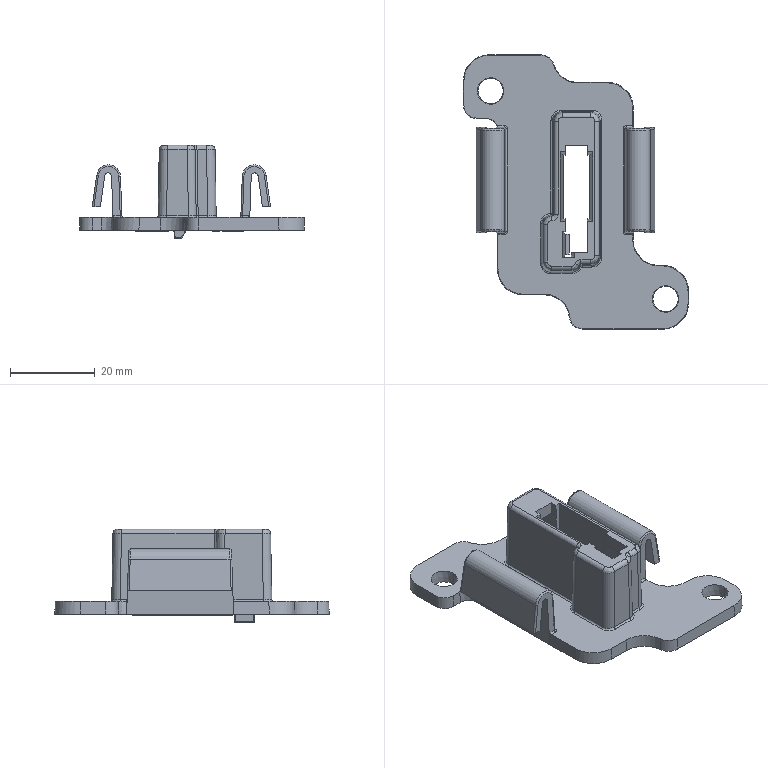Part | STEP file | 64534459 | 3 solids | 1455 faces | box 53 x 64.6 x 22 mm | volume 11629 mm3 | plane 849 | other 498 | cylinder 72 | spline 25 | sphere 7 | cone 4 | commonest cylinder face diameters 0.8 x20 0.4 x17 12 x8 2 x6 4 x6 0.32 x3